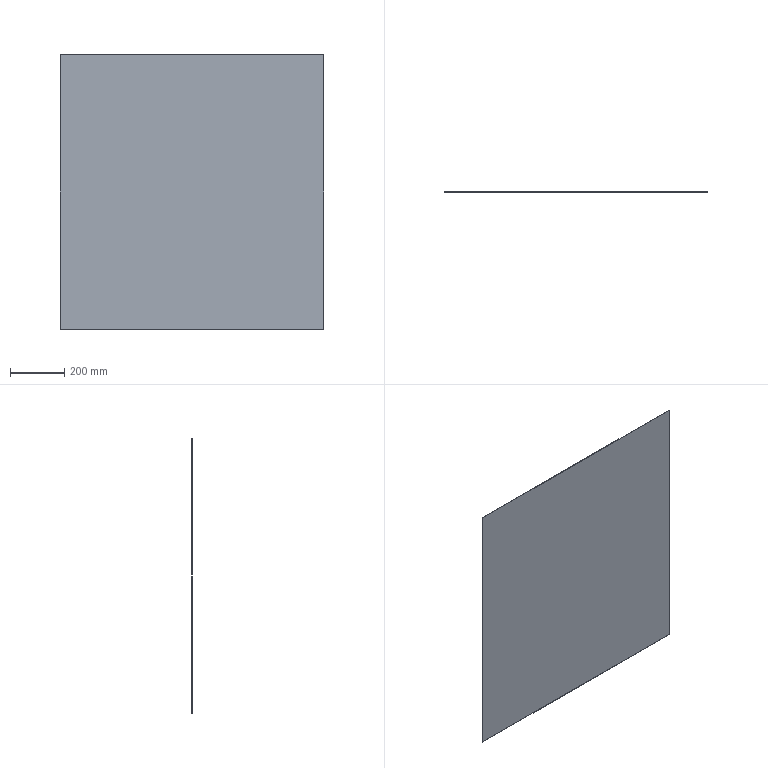Part | STEP file | Guide wheel mechanism revised.sldasm-Part-11 | 1 solid | 6 faces | box 972.42 x 1.2 x 1012 mm | volume 1181397 mm3 | plane 6
STEP:
#1=CARTESIAN_POINT('',(-486.21,1970.01,-506.21));
#2=VERTEX_POINT('',#1);
#3=CARTESIAN_POINT('',(-486.21,1970.01,506.21));
#4=VERTEX_POINT('',#3);
#5=CARTESIAN_POINT('',(-486.21,1970.01,506.21));
#6=DIRECTION('',(0.,0.,1.));
#7=VECTOR('',#6,1000.);
#8=LINE('',#5,#7);
#9=EDGE_CURVE('',#2,#4,#8,.T.);
#10=ORIENTED_EDGE('',*,*,#9,.T.);
#11=CARTESIAN_POINT('',(-486.21,1971.21,506.21));
#12=VERTEX_POINT('',#11);
#13=CARTESIAN_POINT('',(-486.21,1971.21,506.21));
#14=DIRECTION('',(0.,-1.,0.));
#15=VECTOR('',#14,1000.);
#16=LINE('',#13,#15);
#17=EDGE_CURVE('',#12,#4,#16,.T.);
#18=ORIENTED_EDGE('',*,*,#17,.F.);
#19=CARTESIAN_POINT('',(-486.21,1971.21,-506.21));
#20=VERTEX_POINT('',#19);
#21=CARTESIAN_POINT('',(-486.21,1971.21,506.21));
#22=DIRECTION('',(0.,0.,1.));
#23=VECTOR('',#22,1000.);
#24=LINE('',#21,#23);
#25=EDGE_CURVE('',#20,#12,#24,.T.);
#26=ORIENTED_EDGE('',*,*,#25,.F.);
#27=CARTESIAN_POINT('',(-486.21,1971.21,-506.21));
#28=DIRECTION('',(0.,-1.,0.));
#29=VECTOR('',#28,1000.);
#30=LINE('',#27,#29);
#31=EDGE_CURVE('',#20,#2,#30,.T.);
#32=ORIENTED_EDGE('',*,*,#31,.T.);
#33=EDGE_LOOP('',(#10,#18,#26,#32));
#34=FACE_OUTER_BOUND('',#33,.T.);
#35=CARTESIAN_POINT('',(-486.21,1971.21,506.21));
#36=DIRECTION('',(1.,0.,0.));
#37=DIRECTION('',(0.,0.,-1.));
#38=AXIS2_PLACEMENT_3D('',#35,#36,#37);
#39=PLANE('',#38);
#40=ADVANCED_FACE('',(#34),#39,.F.);
#41=CARTESIAN_POINT('',(486.21,1970.01,506.21));
#42=VERTEX_POINT('',#41);
#43=CARTESIAN_POINT('',(486.21,1970.01,506.21));
#44=DIRECTION('',(1.,0.,0.));
#45=VECTOR('',#44,1000.);
#46=LINE('',#43,#45);
#47=EDGE_CURVE('',#4,#42,#46,.T.);
#48=ORIENTED_EDGE('',*,*,#47,.T.);
#49=CARTESIAN_POINT('',(486.21,1971.21,506.21));
#50=VERTEX_POINT('',#49);
#51=CARTESIAN_POINT('',(486.21,1971.21,506.21));
#52=DIRECTION('',(0.,-1.,0.));
#53=VECTOR('',#52,1000.);
#54=LINE('',#51,#53);
#55=EDGE_CURVE('',#50,#42,#54,.T.);
#56=ORIENTED_EDGE('',*,*,#55,.F.);
#57=CARTESIAN_POINT('',(486.21,1971.21,506.21));
#58=DIRECTION('',(1.,0.,0.));
#59=VECTOR('',#58,1000.);
#60=LINE('',#57,#59);
#61=EDGE_CURVE('',#12,#50,#60,.T.);
#62=ORIENTED_EDGE('',*,*,#61,.F.);
#63=ORIENTED_EDGE('',*,*,#17,.T.);
#64=EDGE_LOOP('',(#48,#56,#62,#63));
#65=FACE_OUTER_BOUND('',#64,.T.);
#66=CARTESIAN_POINT('',(486.21,1971.21,506.21));
#67=DIRECTION('',(0.,0.,-1.));
#68=DIRECTION('',(-1.,0.,0.));
#69=AXIS2_PLACEMENT_3D('',#66,#67,#68);
#70=PLANE('',#69);
#71=ADVANCED_FACE('',(#65),#70,.F.);
#72=CARTESIAN_POINT('',(486.21,1970.01,-506.21));
#73=VERTEX_POINT('',#72);
#74=CARTESIAN_POINT('',(486.21,1970.01,506.21));
#75=DIRECTION('',(0.,0.,-1.));
#76=VECTOR('',#75,1000.);
#77=LINE('',#74,#76);
#78=EDGE_CURVE('',#42,#73,#77,.T.);
#79=ORIENTED_EDGE('',*,*,#78,.T.);
#80=CARTESIAN_POINT('',(486.21,1971.21,-506.21));
#81=VERTEX_POINT('',#80);
#82=CARTESIAN_POINT('',(486.21,1971.21,-506.21));
#83=DIRECTION('',(0.,-1.,0.));
#84=VECTOR('',#83,1000.);
#85=LINE('',#82,#84);
#86=EDGE_CURVE('',#81,#73,#85,.T.);
#87=ORIENTED_EDGE('',*,*,#86,.F.);
#88=CARTESIAN_POINT('',(486.21,1971.21,506.21));
#89=DIRECTION('',(0.,0.,-1.));
#90=VECTOR('',#89,1000.);
#91=LINE('',#88,#90);
#92=EDGE_CURVE('',#50,#81,#91,.T.);
#93=ORIENTED_EDGE('',*,*,#92,.F.);
#94=ORIENTED_EDGE('',*,*,#55,.T.);
#95=EDGE_LOOP('',(#79,#87,#93,#94));
#96=FACE_OUTER_BOUND('',#95,.T.);
#97=CARTESIAN_POINT('',(486.21,1971.21,506.21));
#98=DIRECTION('',(-1.,0.,0.));
#99=DIRECTION('',(0.,0.,1.));
#100=AXIS2_PLACEMENT_3D('',#97,#98,#99);
#101=PLANE('',#100);
#102=ADVANCED_FACE('',(#96),#101,.F.);
#103=CARTESIAN_POINT('',(486.21,1970.01,-506.21));
#104=DIRECTION('',(-1.,0.,0.));
#105=VECTOR('',#104,1000.);
#106=LINE('',#103,#105);
#107=EDGE_CURVE('',#73,#2,#106,.T.);
#108=ORIENTED_EDGE('',*,*,#107,.T.);
#109=ORIENTED_EDGE('',*,*,#31,.F.);
#110=CARTESIAN_POINT('',(486.21,1971.21,-506.21));
#111=DIRECTION('',(-1.,0.,0.));
#112=VECTOR('',#111,1000.);
#113=LINE('',#110,#112);
#114=EDGE_CURVE('',#81,#20,#113,.T.);
#115=ORIENTED_EDGE('',*,*,#114,.F.);
#116=ORIENTED_EDGE('',*,*,#86,.T.);
#117=EDGE_LOOP('',(#108,#109,#115,#116));
#118=FACE_OUTER_BOUND('',#117,.T.);
#119=CARTESIAN_POINT('',(486.21,1971.21,-506.21));
#120=DIRECTION('',(0.,0.,1.));
#121=DIRECTION('',(1.,0.,0.));
#122=AXIS2_PLACEMENT_3D('',#119,#120,#121);
#123=PLANE('',#122);
#124=ADVANCED_FACE('',(#118),#123,.F.);
#125=ORIENTED_EDGE('',*,*,#25,.T.);
#126=ORIENTED_EDGE('',*,*,#61,.T.);
#127=ORIENTED_EDGE('',*,*,#92,.T.);
#128=ORIENTED_EDGE('',*,*,#114,.T.);
#129=EDGE_LOOP('',(#125,#126,#127,#128));
#130=FACE_OUTER_BOUND('',#129,.T.);
#131=CARTESIAN_POINT('',(0.,1971.21,0.));
#132=DIRECTION('',(0.,1.,0.));
#133=DIRECTION('',(0.,0.,1.));
#134=AXIS2_PLACEMENT_3D('',#131,#132,#133);
#135=PLANE('',#134);
#136=ADVANCED_FACE('',(#130),#135,.T.);
#137=ORIENTED_EDGE('',*,*,#9,.F.);
#138=ORIENTED_EDGE('',*,*,#107,.F.);
#139=ORIENTED_EDGE('',*,*,#78,.F.);
#140=ORIENTED_EDGE('',*,*,#47,.F.);
#141=EDGE_LOOP('',(#137,#138,#139,#140));
#142=FACE_OUTER_BOUND('',#141,.T.);
#143=CARTESIAN_POINT('',(0.,1970.01,0.));
#144=DIRECTION('',(0.,1.,0.));
#145=DIRECTION('',(0.,0.,1.));
#146=AXIS2_PLACEMENT_3D('',#143,#144,#145);
#147=PLANE('',#146);
#148=ADVANCED_FACE('',(#142),#147,.F.);
#149=CLOSED_SHELL('',(#40,#71,#102,#124,#136,#148));
#150=MANIFOLD_SOLID_BREP('',#149);
#151=CARTESIAN_POINT('',(0.,0.,0.));
#152=DIRECTION('',(0.,0.,1.));
#153=DIRECTION('',(1.,0.,0.));
#154=AXIS2_PLACEMENT_3D('',#151,#152,#153);
#155=(LENGTH_UNIT()NAMED_UNIT(*)SI_UNIT(.MILLI.,.METRE.));
#156=UNCERTAINTY_MEASURE_WITH_UNIT(LENGTH_MEASURE(0.00001),#155,'','');
#157=(NAMED_UNIT(*)PLANE_ANGLE_UNIT()SI_UNIT($,.RADIAN.));
#158=(NAMED_UNIT(*)SI_UNIT($,.STERADIAN.)SOLID_ANGLE_UNIT());
#159=(GEOMETRIC_REPRESENTATION_CONTEXT(3)GLOBAL_UNCERTAINTY_ASSIGNED_CONTEXT((#156))GLOBAL_UNIT_ASSIGNED_CONTEXT((#155,#157,#158))REPRESENTATION_CONTEXT('',''));
#160=ADVANCED_BREP_SHAPE_REPRESENTATION('',(#150,#154),#159);